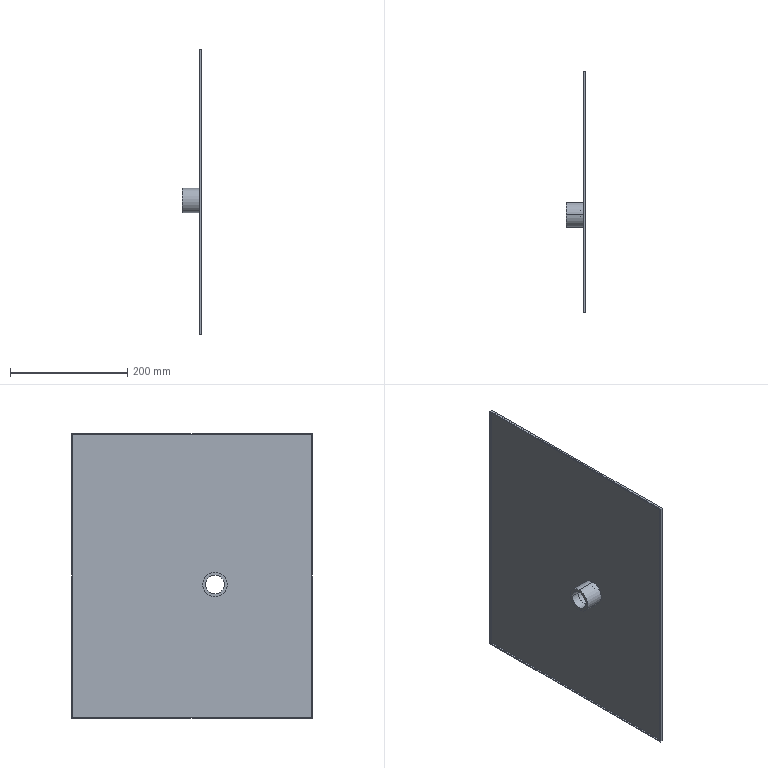Part | STEP file | 09-29 Cover lid plate | 1 solid | 25 faces | box 34 x 410 x 485 mm | volume 320588 mm3 | plane 15 | cylinder 10 | commonest cylinder face diameters 35 x4 32 x2 37.8 x2 42 x2